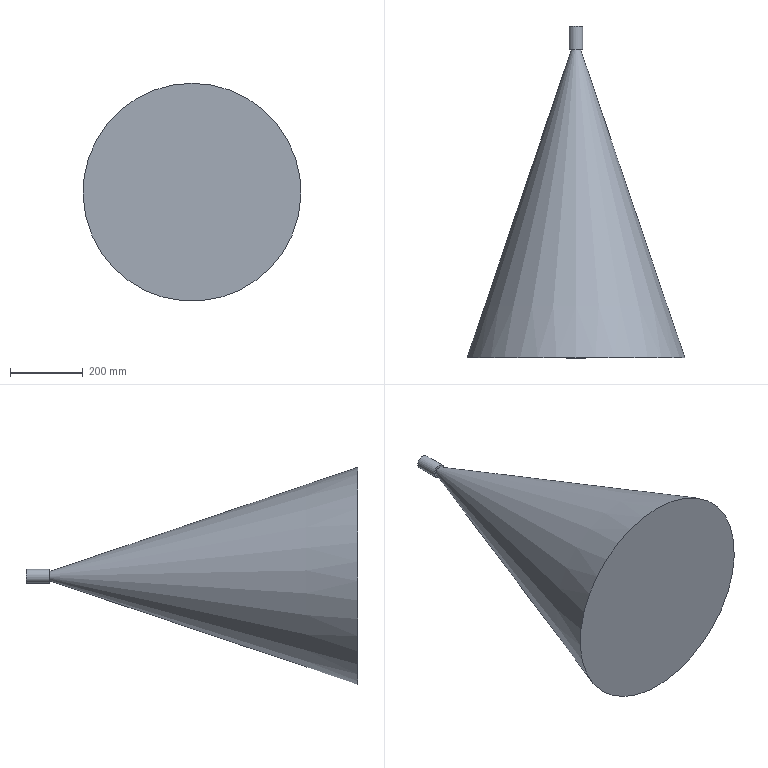Part | NX | 1 solid | 5 faces | box 600 x 914 x 600 mm | volume 83660219 mm3 | plane 3 | cylinder 1 | cone 1 | commonest cylinder face diameters 38 x1
STEP:
#1=CARTESIAN_POINT('',(0.,0.,19.));
#2=VERTEX_POINT('',#1);
#3=CARTESIAN_POINT('',(0.,0.,0.));
#4=DIRECTION('',(0.,1.,0.));
#5=DIRECTION('',(0.,0.,1.));
#6=AXIS2_PLACEMENT_3D('',#3,#4,#5);
#7=CIRCLE('',#6,19.);
#8=EDGE_CURVE('',#2,#2,#7,.T.);
#9=ORIENTED_EDGE('',*,*,#8,.F.);
#10=EDGE_LOOP('',(#9));
#11=FACE_BOUND('',#10,.T.);
#12=CARTESIAN_POINT('',(0.,0.,12.5));
#13=VERTEX_POINT('',#12);
#14=CARTESIAN_POINT('',(0.,0.,0.));
#15=DIRECTION('',(0.,1.,0.));
#16=DIRECTION('',(0.,0.,1.));
#17=AXIS2_PLACEMENT_3D('',#14,#15,#16);
#18=CIRCLE('',#17,12.5);
#19=EDGE_CURVE('',#13,#13,#18,.F.);
#20=ORIENTED_EDGE('',*,*,#19,.F.);
#21=EDGE_LOOP('',(#20));
#22=FACE_BOUND('',#21,.T.);
#23=CARTESIAN_POINT('',(0.,0.,0.));
#24=DIRECTION('',(0.,1.,0.));
#25=DIRECTION('',(0.,0.,1.));
#26=AXIS2_PLACEMENT_3D('',#23,#24,#25);
#27=PLANE('',#26);
#28=ADVANCED_FACE('',(#11,#22),#27,.F.);
#29=CARTESIAN_POINT('',(0.,64.,19.));
#30=VERTEX_POINT('',#29);
#31=CARTESIAN_POINT('',(0.,64.,0.));
#32=DIRECTION('',(0.,1.,0.));
#33=DIRECTION('',(0.,0.,1.));
#34=AXIS2_PLACEMENT_3D('',#31,#32,#33);
#35=CIRCLE('',#34,19.);
#36=EDGE_CURVE('',#30,#30,#35,.T.);
#37=ORIENTED_EDGE('',*,*,#36,.F.);
#38=EDGE_LOOP('',(#37));
#39=FACE_BOUND('',#38,.T.);
#40=ORIENTED_EDGE('',*,*,#8,.T.);
#41=EDGE_LOOP('',(#40));
#42=FACE_BOUND('',#41,.T.);
#43=CARTESIAN_POINT('',(0.,64.,0.));
#44=DIRECTION('',(0.,-1.,0.));
#45=DIRECTION('',(0.,0.,-1.));
#46=AXIS2_PLACEMENT_3D('',#43,#44,#45);
#47=CYLINDRICAL_SURFACE('',#46,19.);
#48=ADVANCED_FACE('',(#39,#42),#47,.T.);
#49=ORIENTED_EDGE('',*,*,#36,.T.);
#50=EDGE_LOOP('',(#49));
#51=FACE_BOUND('',#50,.T.);
#52=CARTESIAN_POINT('',(0.,64.,0.));
#53=DIRECTION('',(0.,1.,0.));
#54=DIRECTION('',(0.,0.,1.));
#55=AXIS2_PLACEMENT_3D('',#52,#53,#54);
#56=PLANE('',#55);
#57=ADVANCED_FACE('',(#51),#56,.T.);
#58=ORIENTED_EDGE('',*,*,#19,.T.);
#59=EDGE_LOOP('',(#58));
#60=FACE_BOUND('',#59,.T.);
#61=CARTESIAN_POINT('',(0.,-850.,300.));
#62=VERTEX_POINT('',#61);
#63=CARTESIAN_POINT('',(0.,-850.,0.));
#64=DIRECTION('',(0.,1.,0.));
#65=DIRECTION('',(0.,0.,1.));
#66=AXIS2_PLACEMENT_3D('',#63,#64,#65);
#67=CIRCLE('',#66,300.);
#68=EDGE_CURVE('',#62,#62,#67,.T.);
#69=ORIENTED_EDGE('',*,*,#68,.T.);
#70=EDGE_LOOP('',(#69));
#71=FACE_BOUND('',#70,.T.);
#72=CARTESIAN_POINT('',(0.,-850.,0.));
#73=DIRECTION('',(0.,-1.,0.));
#74=DIRECTION('',(0.,0.,-1.));
#75=AXIS2_PLACEMENT_3D('',#72,#73,#74);
#76=CONICAL_SURFACE('',#75,300.,0.3262);
#77=ADVANCED_FACE('',(#60,#71),#76,.T.);
#78=ORIENTED_EDGE('',*,*,#68,.F.);
#79=EDGE_LOOP('',(#78));
#80=FACE_BOUND('',#79,.T.);
#81=CARTESIAN_POINT('',(300.,-850.,0.));
#82=DIRECTION('',(0.,1.,0.));
#83=DIRECTION('',(0.,0.,1.));
#84=AXIS2_PLACEMENT_3D('',#81,#82,#83);
#85=PLANE('',#84);
#86=ADVANCED_FACE('',(#80),#85,.F.);
#87=CLOSED_SHELL('',(#28,#48,#57,#77,#86));
#88=MANIFOLD_SOLID_BREP('',#87);
#89=(LENGTH_UNIT()NAMED_UNIT(*)SI_UNIT(.MILLI.,.METRE.));
#90=UNCERTAINTY_MEASURE_WITH_UNIT(LENGTH_MEASURE(0.00001),#89,'','');
#91=(NAMED_UNIT(*)PLANE_ANGLE_UNIT()SI_UNIT($,.RADIAN.));
#92=(NAMED_UNIT(*)SI_UNIT($,.STERADIAN.)SOLID_ANGLE_UNIT());
#93=(GEOMETRIC_REPRESENTATION_CONTEXT(3)GLOBAL_UNCERTAINTY_ASSIGNED_CONTEXT((#90))GLOBAL_UNIT_ASSIGNED_CONTEXT((#89,#91,#92))REPRESENTATION_CONTEXT('',''));
#94=ADVANCED_BREP_SHAPE_REPRESENTATION('',(#88),#93);